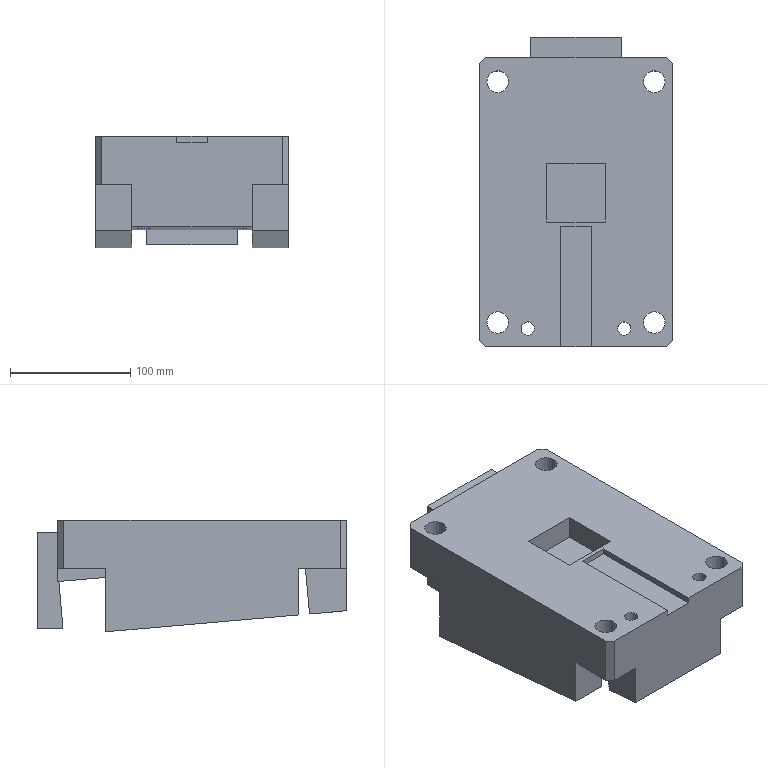Part | NX | features solid 2 | 1 solid | 57 faces | box 160 x 257 x 92.67 mm | volume 2105818 mm3 | plane 47 | cylinder 10 | commonest cylinder face diameters 18 x4 26 x4 11 x2